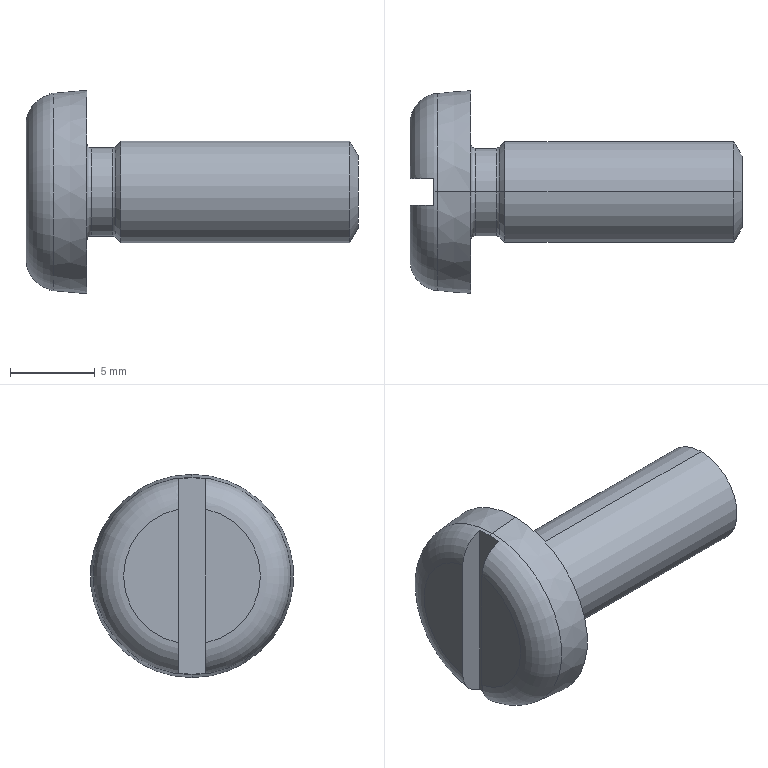Part | SolidWorks | features Fillet 2, ICE 1, LPattern 1, RevCut 1, Revolution 1 | 1 solid | 23 faces | box 19.6 x 12 x 12 mm | volume 779.516 mm3 | plane 7 | cone 6 | torus 6 | cylinder 4 | commonest cylinder face diameters 5.196 x2 6 x2
STEP:
#1=CARTESIAN_POINT('',(19.6,0.,2.134));
#2=VERTEX_POINT('',#1);
#3=CARTESIAN_POINT('',(19.6,0.,-2.134));
#4=VERTEX_POINT('',#3);
#5=CARTESIAN_POINT('',(19.6,0.,0.));
#6=DIRECTION('',(-1.,0.,0.));
#7=DIRECTION('',(0.,0.,1.));
#8=AXIS2_PLACEMENT_3D('',#5,#6,#7);
#9=CIRCLE('',#8,2.134);
#10=EDGE_CURVE('',#2,#4,#9,.T.);
#11=ORIENTED_EDGE('',*,*,#10,.T.);
#12=CARTESIAN_POINT('',(19.105,0.,-3.));
#13=VERTEX_POINT('',#12);
#14=CARTESIAN_POINT('',(19.105,0.,-3.));
#15=DIRECTION('',(-0.4959,0.,-0.8684));
#16=VECTOR('',#15,1000.);
#17=LINE('',#14,#16);
#18=EDGE_CURVE('',#4,#13,#17,.T.);
#19=ORIENTED_EDGE('',*,*,#18,.T.);
#20=CARTESIAN_POINT('',(19.105,0.,3.));
#21=VERTEX_POINT('',#20);
#22=CARTESIAN_POINT('',(19.105,0.,0.));
#23=DIRECTION('',(-1.,0.,0.));
#24=DIRECTION('',(0.,0.,1.));
#25=AXIS2_PLACEMENT_3D('',#22,#23,#24);
#26=CIRCLE('',#25,3.);
#27=EDGE_CURVE('',#21,#13,#26,.T.);
#28=ORIENTED_EDGE('',*,*,#27,.F.);
#29=CARTESIAN_POINT('',(19.105,0.,3.));
#30=DIRECTION('',(-0.4959,0.,0.8684));
#31=VECTOR('',#30,1000.);
#32=LINE('',#29,#31);
#33=EDGE_CURVE('',#2,#21,#32,.T.);
#34=ORIENTED_EDGE('',*,*,#33,.F.);
#35=EDGE_LOOP('',(#11,#19,#28,#34));
#36=FACE_OUTER_BOUND('',#35,.T.);
#37=CARTESIAN_POINT('',(19.105,0.,0.));
#38=DIRECTION('',(-1.,0.,0.));
#39=DIRECTION('',(0.,0.,1.));
#40=AXIS2_PLACEMENT_3D('',#37,#38,#39);
#41=CONICAL_SURFACE('',#40,3.,1.052);
#42=ADVANCED_FACE('',(#36),#41,.T.);
#43=CARTESIAN_POINT('',(3.6,0.,-2.848));
#44=VERTEX_POINT('',#43);
#45=CARTESIAN_POINT('',(3.6,0.,2.848));
#46=VERTEX_POINT('',#45);
#47=CARTESIAN_POINT('',(3.6,0.,0.));
#48=DIRECTION('',(-1.,0.,0.));
#49=DIRECTION('',(0.,0.,1.));
#50=AXIS2_PLACEMENT_3D('',#47,#48,#49);
#51=CIRCLE('',#50,2.848);
#52=EDGE_CURVE('',#44,#46,#51,.T.);
#53=ORIENTED_EDGE('',*,*,#52,.F.);
#54=CARTESIAN_POINT('',(3.85,0.,-2.598));
#55=VERTEX_POINT('',#54);
#56=CARTESIAN_POINT('',(3.85,0.,-2.848));
#57=DIRECTION('',(0.,1.,0.));
#58=DIRECTION('',(0.,0.,1.));
#59=AXIS2_PLACEMENT_3D('',#56,#57,#58);
#60=CIRCLE('',#59,0.25);
#61=EDGE_CURVE('',#44,#55,#60,.T.);
#62=ORIENTED_EDGE('',*,*,#61,.T.);
#63=CARTESIAN_POINT('',(3.85,0.,2.598));
#64=VERTEX_POINT('',#63);
#65=CARTESIAN_POINT('',(3.85,0.,0.));
#66=DIRECTION('',(1.,0.,0.));
#67=DIRECTION('',(0.,0.,1.));
#68=AXIS2_PLACEMENT_3D('',#65,#66,#67);
#69=CIRCLE('',#68,2.598);
#70=EDGE_CURVE('',#64,#55,#69,.T.);
#71=ORIENTED_EDGE('',*,*,#70,.F.);
#72=CARTESIAN_POINT('',(3.85,0.,2.848));
#73=DIRECTION('',(0.,-1.,0.));
#74=DIRECTION('',(0.,0.,-1.));
#75=AXIS2_PLACEMENT_3D('',#72,#73,#74);
#76=CIRCLE('',#75,0.25);
#77=EDGE_CURVE('',#46,#64,#76,.T.);
#78=ORIENTED_EDGE('',*,*,#77,.F.);
#79=EDGE_LOOP('',(#53,#62,#71,#78));
#80=FACE_OUTER_BOUND('',#79,.T.);
#81=CARTESIAN_POINT('',(3.85,0.,0.));
#82=DIRECTION('',(-1.,0.,0.));
#83=DIRECTION('',(0.,0.,1.));
#84=AXIS2_PLACEMENT_3D('',#81,#82,#83);
#85=TOROIDAL_SURFACE('',#84,2.848,0.25);
#86=ADVANCED_FACE('',(#80),#85,.F.);
#87=CARTESIAN_POINT('',(5.094,0.,-2.598));
#88=VERTEX_POINT('',#87);
#89=CARTESIAN_POINT('',(5.094,0.,2.598));
#90=VERTEX_POINT('',#89);
#91=CARTESIAN_POINT('',(5.094,0.,0.));
#92=DIRECTION('',(-1.,0.,0.));
#93=DIRECTION('',(0.,0.,1.));
#94=AXIS2_PLACEMENT_3D('',#91,#92,#93);
#95=CIRCLE('',#94,2.598);
#96=EDGE_CURVE('',#88,#90,#95,.T.);
#97=ORIENTED_EDGE('',*,*,#96,.F.);
#98=CARTESIAN_POINT('',(5.271,0.,-2.671));
#99=VERTEX_POINT('',#98);
#100=CARTESIAN_POINT('',(5.094,0.,-2.848));
#101=DIRECTION('',(0.,1.,0.));
#102=DIRECTION('',(0.,0.,1.));
#103=AXIS2_PLACEMENT_3D('',#100,#101,#102);
#104=CIRCLE('',#103,0.25);
#105=EDGE_CURVE('',#88,#99,#104,.T.);
#106=ORIENTED_EDGE('',*,*,#105,.T.);
#107=CARTESIAN_POINT('',(5.271,0.,2.671));
#108=VERTEX_POINT('',#107);
#109=CARTESIAN_POINT('',(5.271,0.,0.));
#110=DIRECTION('',(1.,0.,0.));
#111=DIRECTION('',(0.,0.,-1.));
#112=AXIS2_PLACEMENT_3D('',#109,#110,#111);
#113=CIRCLE('',#112,2.671);
#114=EDGE_CURVE('',#108,#99,#113,.T.);
#115=ORIENTED_EDGE('',*,*,#114,.F.);
#116=CARTESIAN_POINT('',(5.094,0.,2.848));
#117=DIRECTION('',(0.,-1.,0.));
#118=DIRECTION('',(0.,0.,-1.));
#119=AXIS2_PLACEMENT_3D('',#116,#117,#118);
#120=CIRCLE('',#119,0.25);
#121=EDGE_CURVE('',#90,#108,#120,.T.);
#122=ORIENTED_EDGE('',*,*,#121,.F.);
#123=EDGE_LOOP('',(#97,#106,#115,#122));
#124=FACE_OUTER_BOUND('',#123,.T.);
#125=CARTESIAN_POINT('',(5.094,0.,0.));
#126=DIRECTION('',(-1.,0.,0.));
#127=DIRECTION('',(0.,0.,1.));
#128=AXIS2_PLACEMENT_3D('',#125,#126,#127);
#129=TOROIDAL_SURFACE('',#128,2.848,0.25);
#130=ADVANCED_FACE('',(#124),#129,.F.);
#131=CARTESIAN_POINT('',(1.643,0.,-5.829));
#132=VERTEX_POINT('',#131);
#133=CARTESIAN_POINT('',(1.643,0.,5.829));
#134=VERTEX_POINT('',#133);
#135=CARTESIAN_POINT('',(1.643,0.,0.));
#136=DIRECTION('',(1.,0.,0.));
#137=DIRECTION('',(0.,0.,1.));
#138=AXIS2_PLACEMENT_3D('',#135,#136,#137);
#139=CIRCLE('',#138,5.829);
#140=EDGE_CURVE('',#132,#134,#139,.T.);
#141=ORIENTED_EDGE('',*,*,#140,.T.);
#142=CARTESIAN_POINT('',(3.6,0.,6.));
#143=VERTEX_POINT('',#142);
#144=CARTESIAN_POINT('',(3.6,0.,6.));
#145=DIRECTION('',(0.9962,0.,0.08716));
#146=VECTOR('',#145,1000.);
#147=LINE('',#144,#146);
#148=EDGE_CURVE('',#134,#143,#147,.T.);
#149=ORIENTED_EDGE('',*,*,#148,.T.);
#150=CARTESIAN_POINT('',(3.6,0.,-6.));
#151=VERTEX_POINT('',#150);
#152=CARTESIAN_POINT('',(3.6,0.,0.));
#153=DIRECTION('',(-1.,0.,0.));
#154=DIRECTION('',(0.,0.,1.));
#155=AXIS2_PLACEMENT_3D('',#152,#153,#154);
#156=CIRCLE('',#155,6.);
#157=EDGE_CURVE('',#143,#151,#156,.T.);
#158=ORIENTED_EDGE('',*,*,#157,.T.);
#159=CARTESIAN_POINT('',(3.6,0.,-6.));
#160=DIRECTION('',(0.9962,0.,-0.08716));
#161=VECTOR('',#160,1000.);
#162=LINE('',#159,#161);
#163=EDGE_CURVE('',#132,#151,#162,.T.);
#164=ORIENTED_EDGE('',*,*,#163,.F.);
#165=EDGE_LOOP('',(#141,#149,#158,#164));
#166=FACE_OUTER_BOUND('',#165,.T.);
#167=CARTESIAN_POINT('',(3.6,0.,0.));
#168=DIRECTION('',(1.,0.,0.));
#169=DIRECTION('',(0.,0.,-1.));
#170=AXIS2_PLACEMENT_3D('',#167,#168,#169);
#171=CONICAL_SURFACE('',#170,6.,0.08727);
#172=ADVANCED_FACE('',(#166),#171,.T.);
#173=CARTESIAN_POINT('',(5.094,0.,0.));
#174=DIRECTION('',(-1.,0.,0.));
#175=DIRECTION('',(0.,0.,1.));
#176=AXIS2_PLACEMENT_3D('',#173,#174,#175);
#177=CIRCLE('',#176,2.598);
#178=EDGE_CURVE('',#90,#88,#177,.T.);
#179=ORIENTED_EDGE('',*,*,#178,.T.);
#180=CARTESIAN_POINT('',(-3.442,0.,-2.598));
#181=DIRECTION('',(-1.,0.,0.));
#182=VECTOR('',#181,1000.);
#183=LINE('',#180,#182);
#184=EDGE_CURVE('',#88,#55,#183,.T.);
#185=ORIENTED_EDGE('',*,*,#184,.T.);
#186=CARTESIAN_POINT('',(3.85,0.,0.));
#187=DIRECTION('',(1.,0.,0.));
#188=DIRECTION('',(0.,0.,1.));
#189=AXIS2_PLACEMENT_3D('',#186,#187,#188);
#190=CIRCLE('',#189,2.598);
#191=EDGE_CURVE('',#55,#64,#190,.T.);
#192=ORIENTED_EDGE('',*,*,#191,.T.);
#193=CARTESIAN_POINT('',(-3.442,0.,2.598));
#194=DIRECTION('',(-1.,0.,0.));
#195=VECTOR('',#194,1000.);
#196=LINE('',#193,#195);
#197=EDGE_CURVE('',#90,#64,#196,.T.);
#198=ORIENTED_EDGE('',*,*,#197,.F.);
#199=EDGE_LOOP('',(#179,#185,#192,#198));
#200=FACE_OUTER_BOUND('',#199,.T.);
#201=CARTESIAN_POINT('',(-3.442,0.,0.));
#202=DIRECTION('',(-1.,0.,0.));
#203=DIRECTION('',(0.,0.,1.));
#204=AXIS2_PLACEMENT_3D('',#201,#202,#203);
#205=CYLINDRICAL_SURFACE('',#204,2.598);
#206=ADVANCED_FACE('',(#200),#205,.T.);
#207=CARTESIAN_POINT('',(5.271,0.,0.));
#208=DIRECTION('',(1.,0.,0.));
#209=DIRECTION('',(0.,0.,-1.));
#210=AXIS2_PLACEMENT_3D('',#207,#208,#209);
#211=CIRCLE('',#210,2.671);
#212=EDGE_CURVE('',#99,#108,#211,.T.);
#213=ORIENTED_EDGE('',*,*,#212,.T.);
#214=CARTESIAN_POINT('',(5.6,0.,3.));
#215=VERTEX_POINT('',#214);
#216=CARTESIAN_POINT('',(5.6,0.,3.));
#217=DIRECTION('',(0.7071,0.,0.7071));
#218=VECTOR('',#217,1000.);
#219=LINE('',#216,#218);
#220=EDGE_CURVE('',#108,#215,#219,.T.);
#221=ORIENTED_EDGE('',*,*,#220,.T.);
#222=CARTESIAN_POINT('',(5.6,0.,-3.));
#223=VERTEX_POINT('',#222);
#224=CARTESIAN_POINT('',(5.6,0.,0.));
#225=DIRECTION('',(-1.,0.,0.));
#226=DIRECTION('',(0.,0.,1.));
#227=AXIS2_PLACEMENT_3D('',#224,#225,#226);
#228=CIRCLE('',#227,3.);
#229=EDGE_CURVE('',#215,#223,#228,.T.);
#230=ORIENTED_EDGE('',*,*,#229,.T.);
#231=CARTESIAN_POINT('',(5.6,0.,-3.));
#232=DIRECTION('',(0.7071,0.,-0.7071));
#233=VECTOR('',#232,1000.);
#234=LINE('',#231,#233);
#235=EDGE_CURVE('',#99,#223,#234,.T.);
#236=ORIENTED_EDGE('',*,*,#235,.F.);
#237=EDGE_LOOP('',(#213,#221,#230,#236));
#238=FACE_OUTER_BOUND('',#237,.T.);
#239=CARTESIAN_POINT('',(5.6,0.,0.));
#240=DIRECTION('',(1.,0.,0.));
#241=DIRECTION('',(0.,0.,-1.));
#242=AXIS2_PLACEMENT_3D('',#239,#240,#241);
#243=CONICAL_SURFACE('',#242,3.,0.7854);
#244=ADVANCED_FACE('',(#238),#243,.T.);
#245=CARTESIAN_POINT('',(1.4,0.8,5.735));
#246=VERTEX_POINT('',#245);
#247=CARTESIAN_POINT('',(1.4,0.,5.791));
#248=VERTEX_POINT('',#247);
#249=CARTESIAN_POINT('',(1.4,0.,0.));
#250=DIRECTION('',(1.,0.,0.));
#251=DIRECTION('',(0.,0.,1.));
#252=AXIS2_PLACEMENT_3D('',#249,#250,#251);
#253=CIRCLE('',#252,5.791);
#254=EDGE_CURVE('',#246,#248,#253,.T.);
#255=ORIENTED_EDGE('',*,*,#254,.T.);
#256=CARTESIAN_POINT('',(1.8,0.,4.036));
#257=DIRECTION('',(0.,1.,0.));
#258=DIRECTION('',(0.,0.,1.));
#259=AXIS2_PLACEMENT_3D('',#256,#257,#258);
#260=CIRCLE('',#259,1.8);
#261=EDGE_CURVE('',#248,#134,#260,.T.);
#262=ORIENTED_EDGE('',*,*,#261,.T.);
#263=ORIENTED_EDGE('',*,*,#140,.F.);
#264=CARTESIAN_POINT('',(1.4,0.,-5.791));
#265=VERTEX_POINT('',#264);
#266=CARTESIAN_POINT('',(1.8,0.,-4.036));
#267=DIRECTION('',(0.,-1.,0.));
#268=DIRECTION('',(0.,0.,-1.));
#269=AXIS2_PLACEMENT_3D('',#266,#267,#268);
#270=CIRCLE('',#269,1.8);
#271=EDGE_CURVE('',#265,#132,#270,.T.);
#272=ORIENTED_EDGE('',*,*,#271,.F.);
#273=CARTESIAN_POINT('',(1.4,0.8,-5.735));
#274=VERTEX_POINT('',#273);
#275=CARTESIAN_POINT('',(1.4,0.,0.));
#276=DIRECTION('',(1.,0.,0.));
#277=DIRECTION('',(0.,0.,1.));
#278=AXIS2_PLACEMENT_3D('',#275,#276,#277);
#279=CIRCLE('',#278,5.791);
#280=EDGE_CURVE('',#265,#274,#279,.T.);
#281=ORIENTED_EDGE('',*,*,#280,.T.);
#282=CARTESIAN_POINT('',(0.,0.8,-3.956));
#283=VERTEX_POINT('',#282);
#284=CARTESIAN_POINT('',(1.4,0.8,-5.735));
#285=CARTESIAN_POINT('',(1.203,0.8,-5.69));
#286=CARTESIAN_POINT('',(1.011,0.8,-5.609));
#287=CARTESIAN_POINT('',(0.6651,0.8,-5.389));
#288=CARTESIAN_POINT('',(0.5144,0.8,-5.251));
#289=CARTESIAN_POINT('',(0.2624,0.8,-4.929));
#290=CARTESIAN_POINT('',(0.1653,0.8,-4.749));
#291=CARTESIAN_POINT('',(0.03314,0.8,-4.362));
#292=CARTESIAN_POINT('',(0.,0.8,-4.16));
#293=CARTESIAN_POINT('',(0.,0.8,-3.956));
#294=B_SPLINE_CURVE_WITH_KNOTS('',3,(#284,#285,#286,#287,#288,#289,#290,#291,#292,#293),.UNSPECIFIED.,.F.,.F.,(4,2,2,2,4),(0.01073,0.01134,0.01195,0.01255,0.01316),.UNSPECIFIED.);
#295=EDGE_CURVE('',#274,#283,#294,.T.);
#296=ORIENTED_EDGE('',*,*,#295,.T.);
#297=CARTESIAN_POINT('',(0.,0.8,3.956));
#298=VERTEX_POINT('',#297);
#299=CARTESIAN_POINT('',(0.,0.,0.));
#300=DIRECTION('',(-1.,0.,0.));
#301=DIRECTION('',(0.,0.,-1.));
#302=AXIS2_PLACEMENT_3D('',#299,#300,#301);
#303=CIRCLE('',#302,4.036);
#304=EDGE_CURVE('',#298,#283,#303,.T.);
#305=ORIENTED_EDGE('',*,*,#304,.F.);
#306=CARTESIAN_POINT('',(0.,0.8,3.956));
#307=CARTESIAN_POINT('',(0.,0.8,4.057));
#308=CARTESIAN_POINT('',(0.008433,0.8,4.16));
#309=CARTESIAN_POINT('',(0.04179,0.8,4.361));
#310=CARTESIAN_POINT('',(0.06654,0.8,4.46));
#311=CARTESIAN_POINT('',(0.165,0.8,4.748));
#312=CARTESIAN_POINT('',(0.2638,0.8,4.931));
#313=CARTESIAN_POINT('',(0.5139,0.8,5.25));
#314=CARTESIAN_POINT('',(0.6679,0.8,5.391));
#315=CARTESIAN_POINT('',(1.01,0.8,5.609));
#316=CARTESIAN_POINT('',(1.202,0.8,5.69));
#317=CARTESIAN_POINT('',(1.4,0.8,5.735));
#318=B_SPLINE_CURVE_WITH_KNOTS('',3,(#306,#307,#308,#309,#310,#311,#312,#313,#314,#315,#316,#317),.UNSPECIFIED.,.F.,.F.,(4,2,2,2,2,4),(0.001725,0.002029,0.002333,0.002941,0.003549,0.004157),.UNSPECIFIED.);
#319=EDGE_CURVE('',#298,#246,#318,.T.);
#320=ORIENTED_EDGE('',*,*,#319,.T.);
#321=EDGE_LOOP('',(#255,#262,#263,#272,#281,#296,#305,#320));
#322=FACE_OUTER_BOUND('',#321,.T.);
#323=CARTESIAN_POINT('',(1.8,0.,0.));
#324=DIRECTION('',(1.,0.,0.));
#325=DIRECTION('',(0.,0.,-1.));
#326=AXIS2_PLACEMENT_3D('',#323,#324,#325);
#327=TOROIDAL_SURFACE('',#326,4.036,1.8);
#328=ADVANCED_FACE('',(#322),#327,.T.);
#329=ORIENTED_EDGE('',*,*,#27,.T.);
#330=CARTESIAN_POINT('',(-3.442,0.,-3.));
#331=DIRECTION('',(-1.,0.,0.));
#332=VECTOR('',#331,1000.);
#333=LINE('',#330,#332);
#334=EDGE_CURVE('',#13,#223,#333,.T.);
#335=ORIENTED_EDGE('',*,*,#334,.T.);
#336=ORIENTED_EDGE('',*,*,#229,.F.);
#337=CARTESIAN_POINT('',(-3.442,0.,3.));
#338=DIRECTION('',(-1.,0.,0.));
#339=VECTOR('',#338,1000.);
#340=LINE('',#337,#339);
#341=EDGE_CURVE('',#21,#215,#340,.T.);
#342=ORIENTED_EDGE('',*,*,#341,.F.);
#343=EDGE_LOOP('',(#329,#335,#336,#342));
#344=FACE_OUTER_BOUND('',#343,.T.);
#345=CARTESIAN_POINT('',(-3.442,0.,0.));
#346=DIRECTION('',(-1.,0.,0.));
#347=DIRECTION('',(0.,0.,1.));
#348=AXIS2_PLACEMENT_3D('',#345,#346,#347);
#349=CYLINDRICAL_SURFACE('',#348,3.);
#350=ADVANCED_FACE('',(#344),#349,.T.);
#351=ORIENTED_EDGE('',*,*,#334,.F.);
#352=CARTESIAN_POINT('',(19.105,0.,0.));
#353=DIRECTION('',(-1.,0.,0.));
#354=DIRECTION('',(0.,0.,1.));
#355=AXIS2_PLACEMENT_3D('',#352,#353,#354);
#356=CIRCLE('',#355,3.);
#357=EDGE_CURVE('',#13,#21,#356,.T.);
#358=ORIENTED_EDGE('',*,*,#357,.T.);
#359=ORIENTED_EDGE('',*,*,#341,.T.);
#360=CARTESIAN_POINT('',(5.6,0.,0.));
#361=DIRECTION('',(-1.,0.,0.));
#362=DIRECTION('',(0.,0.,1.));
#363=AXIS2_PLACEMENT_3D('',#360,#361,#362);
#364=CIRCLE('',#363,3.);
#365=EDGE_CURVE('',#223,#215,#364,.T.);
#366=ORIENTED_EDGE('',*,*,#365,.F.);
#367=EDGE_LOOP('',(#351,#358,#359,#366));
#368=FACE_OUTER_BOUND('',#367,.T.);
#369=CARTESIAN_POINT('',(-3.442,0.,0.));
#370=DIRECTION('',(-1.,0.,0.));
#371=DIRECTION('',(0.,0.,1.));
#372=AXIS2_PLACEMENT_3D('',#369,#370,#371);
#373=CYLINDRICAL_SURFACE('',#372,3.);
#374=ADVANCED_FACE('',(#368),#373,.T.);
#375=CARTESIAN_POINT('',(0.,-0.8,3.956));
#376=VERTEX_POINT('',#375);
#377=CARTESIAN_POINT('',(0.,-0.8,-3.956));
#378=VERTEX_POINT('',#377);
#379=CARTESIAN_POINT('',(0.,-0.8,-6.));
#380=DIRECTION('',(0.,0.,-1.));
#381=VECTOR('',#380,1000.);
#382=LINE('',#379,#381);
#383=EDGE_CURVE('',#376,#378,#382,.T.);
#384=ORIENTED_EDGE('',*,*,#383,.T.);
#385=CARTESIAN_POINT('',(0.,0.,0.));
#386=DIRECTION('',(-1.,0.,0.));
#387=DIRECTION('',(0.,0.,-1.));
#388=AXIS2_PLACEMENT_3D('',#385,#386,#387);
#389=CIRCLE('',#388,4.036);
#390=EDGE_CURVE('',#378,#376,#389,.T.);
#391=ORIENTED_EDGE('',*,*,#390,.T.);
#392=EDGE_LOOP('',(#384,#391));
#393=FACE_OUTER_BOUND('',#392,.T.);
#394=CARTESIAN_POINT('',(0.,5.685,0.));
#395=DIRECTION('',(1.,0.,0.));
#396=DIRECTION('',(0.,0.,-1.));
#397=AXIS2_PLACEMENT_3D('',#394,#395,#396);
#398=PLANE('',#397);
#399=ADVANCED_FACE('',(#393),#398,.F.);
#400=CARTESIAN_POINT('',(0.,0.8,-6.));
#401=DIRECTION('',(0.,0.,1.));
#402=VECTOR('',#401,1000.);
#403=LINE('',#400,#402);
#404=EDGE_CURVE('',#283,#298,#403,.T.);
#405=ORIENTED_EDGE('',*,*,#404,.T.);
#406=ORIENTED_EDGE('',*,*,#304,.T.);
#407=EDGE_LOOP('',(#405,#406));
#408=FACE_OUTER_BOUND('',#407,.T.);
#409=CARTESIAN_POINT('',(0.,5.685,0.));
#410=DIRECTION('',(1.,0.,0.));
#411=DIRECTION('',(0.,0.,-1.));
#412=AXIS2_PLACEMENT_3D('',#409,#410,#411);
#413=PLANE('',#412);
#414=ADVANCED_FACE('',(#408),#413,.F.);
#415=ORIENTED_EDGE('',*,*,#261,.F.);
#416=CARTESIAN_POINT('',(1.4,-0.8,5.735));
#417=VERTEX_POINT('',#416);
#418=CARTESIAN_POINT('',(1.4,0.,0.));
#419=DIRECTION('',(1.,0.,0.));
#420=DIRECTION('',(0.,0.,1.));
#421=AXIS2_PLACEMENT_3D('',#418,#419,#420);
#422=CIRCLE('',#421,5.791);
#423=EDGE_CURVE('',#248,#417,#422,.T.);
#424=ORIENTED_EDGE('',*,*,#423,.T.);
#425=CARTESIAN_POINT('',(1.4,-0.8,5.735));
#426=CARTESIAN_POINT('',(1.2,-0.8,5.689));
#427=CARTESIAN_POINT('',(1.012,-0.8,5.61));
#428=CARTESIAN_POINT('',(0.6661,-0.8,5.389));
#429=CARTESIAN_POINT('',(0.5155,-0.8,5.252));
#430=CARTESIAN_POINT('',(0.2624,-0.8,4.929));
#431=CARTESIAN_POINT('',(0.1658,-0.8,4.75));
#432=CARTESIAN_POINT('',(0.03297,-0.8,4.361));
#433=CARTESIAN_POINT('',(0.,-0.8,4.161));
#434=CARTESIAN_POINT('',(0.,-0.8,3.956));
#435=B_SPLINE_CURVE_WITH_KNOTS('',3,(#425,#426,#427,#428,#429,#430,#431,#432,#433,#434),.UNSPECIFIED.,.F.,.F.,(4,2,2,2,4),(0.00724,0.007848,0.008457,0.009065,0.009674),.UNSPECIFIED.);
#436=EDGE_CURVE('',#417,#376,#435,.T.);
#437=ORIENTED_EDGE('',*,*,#436,.T.);
#438=ORIENTED_EDGE('',*,*,#390,.F.);
#439=CARTESIAN_POINT('',(1.4,-0.8,-5.735));
#440=VERTEX_POINT('',#439);
#441=CARTESIAN_POINT('',(0.,-0.8,-3.956));
#442=CARTESIAN_POINT('',(0.,-0.8,-4.057));
#443=CARTESIAN_POINT('',(0.008456,-0.8,-4.16));
#444=CARTESIAN_POINT('',(0.04165,-0.8,-4.361));
#445=CARTESIAN_POINT('',(0.0663,-0.8,-4.459));
#446=CARTESIAN_POINT('',(0.1319,-0.8,-4.651));
#447=CARTESIAN_POINT('',(0.1733,-0.8,-4.746));
#448=CARTESIAN_POINT('',(0.27,-0.8,-4.925));
#449=CARTESIAN_POINT('',(0.3254,-0.8,-5.009));
#450=CARTESIAN_POINT('',(0.5128,-0.8,-5.249));
#451=CARTESIAN_POINT('',(0.6672,-0.8,-5.39));
#452=CARTESIAN_POINT('',(1.012,-0.8,-5.61));
#453=CARTESIAN_POINT('',(1.201,-0.8,-5.689));
#454=CARTESIAN_POINT('',(1.4,-0.8,-5.735));
#455=B_SPLINE_CURVE_WITH_KNOTS('',3,(#441,#442,#443,#444,#445,#446,#447,#448,#449,#450,#451,#452,#453,#454),.UNSPECIFIED.,.F.,.F.,(4,2,2,2,2,2,4),(0.009623,0.009926,0.01023,0.01053,0.01084,0.01145,0.01205),.UNSPECIFIED.);
#456=EDGE_CURVE('',#378,#440,#455,.T.);
#457=ORIENTED_EDGE('',*,*,#456,.T.);
#458=CARTESIAN_POINT('',(1.4,0.,0.));
#459=DIRECTION('',(1.,0.,0.));
#460=DIRECTION('',(0.,0.,1.));
#461=AXIS2_PLACEMENT_3D('',#458,#459,#460);
#462=CIRCLE('',#461,5.791);
#463=EDGE_CURVE('',#440,#265,#462,.T.);
#464=ORIENTED_EDGE('',*,*,#463,.T.);
#465=ORIENTED_EDGE('',*,*,#271,.T.);
#466=CARTESIAN_POINT('',(1.643,0.,0.));
#467=DIRECTION('',(1.,0.,0.));
#468=DIRECTION('',(0.,0.,1.));
#469=AXIS2_PLACEMENT_3D('',#466,#467,#468);
#470=CIRCLE('',#469,5.829);
#471=EDGE_CURVE('',#134,#132,#470,.T.);
#472=ORIENTED_EDGE('',*,*,#471,.F.);
#473=EDGE_LOOP('',(#415,#424,#437,#438,#457,#464,#465,#472));
#474=FACE_OUTER_BOUND('',#473,.T.);
#475=CARTESIAN_POINT('',(1.8,0.,0.));
#476=DIRECTION('',(1.,0.,0.));
#477=DIRECTION('',(0.,0.,-1.));
#478=AXIS2_PLACEMENT_3D('',#475,#476,#477);
#479=TOROIDAL_SURFACE('',#478,4.036,1.8);
#480=ADVANCED_FACE('',(#474),#479,.T.);
#481=ORIENTED_EDGE('',*,*,#220,.F.);
#482=ORIENTED_EDGE('',*,*,#114,.T.);
#483=ORIENTED_EDGE('',*,*,#235,.T.);
#484=ORIENTED_EDGE('',*,*,#365,.T.);
#485=EDGE_LOOP('',(#481,#482,#483,#484));
#486=FACE_OUTER_BOUND('',#485,.T.);
#487=CARTESIAN_POINT('',(5.6,0.,0.));
#488=DIRECTION('',(1.,0.,0.));
#489=DIRECTION('',(0.,0.,-1.));
#490=AXIS2_PLACEMENT_3D('',#487,#488,#489);
#491=CONICAL_SURFACE('',#490,3.,0.7854);
#492=ADVANCED_FACE('',(#486),#491,.T.);
#493=ORIENTED_EDGE('',*,*,#184,.F.);
#494=ORIENTED_EDGE('',*,*,#96,.T.);
#495=ORIENTED_EDGE('',*,*,#197,.T.);
#496=ORIENTED_EDGE('',*,*,#70,.T.);
#497=EDGE_LOOP('',(#493,#494,#495,#496));
#498=FACE_OUTER_BOUND('',#497,.T.);
#499=CARTESIAN_POINT('',(-3.442,0.,0.));
#500=DIRECTION('',(-1.,0.,0.));
#501=DIRECTION('',(0.,0.,1.));
#502=AXIS2_PLACEMENT_3D('',#499,#500,#501);
#503=CYLINDRICAL_SURFACE('',#502,2.598);
#504=ADVANCED_FACE('',(#498),#503,.T.);
#505=CARTESIAN_POINT('',(3.6,0.,0.));
#506=DIRECTION('',(-1.,0.,0.));
#507=DIRECTION('',(0.,0.,1.));
#508=AXIS2_PLACEMENT_3D('',#505,#506,#507);
#509=CIRCLE('',#508,2.848);
#510=EDGE_CURVE('',#46,#44,#509,.T.);
#511=ORIENTED_EDGE('',*,*,#510,.T.);
#512=ORIENTED_EDGE('',*,*,#52,.T.);
#513=EDGE_LOOP('',(#511,#512));
#514=FACE_BOUND('',#513,.T.);
#515=CARTESIAN_POINT('',(3.6,0.,0.));
#516=DIRECTION('',(-1.,0.,0.));
#517=DIRECTION('',(0.,0.,1.));
#518=AXIS2_PLACEMENT_3D('',#515,#516,#517);
#519=CIRCLE('',#518,6.);
#520=EDGE_CURVE('',#151,#143,#519,.T.);
#521=ORIENTED_EDGE('',*,*,#520,.F.);
#522=ORIENTED_EDGE('',*,*,#157,.F.);
#523=EDGE_LOOP('',(#521,#522));
#524=FACE_OUTER_BOUND('',#523,.T.);
#525=CARTESIAN_POINT('',(3.6,6.,0.));
#526=DIRECTION('',(-1.,0.,0.));
#527=DIRECTION('',(0.,0.,1.));
#528=AXIS2_PLACEMENT_3D('',#525,#526,#527);
#529=PLANE('',#528);
#530=ADVANCED_FACE('',(#514,#524),#529,.F.);
#531=ORIENTED_EDGE('',*,*,#148,.F.);
#532=ORIENTED_EDGE('',*,*,#471,.T.);
#533=ORIENTED_EDGE('',*,*,#163,.T.);
#534=ORIENTED_EDGE('',*,*,#520,.T.);
#535=EDGE_LOOP('',(#531,#532,#533,#534));
#536=FACE_OUTER_BOUND('',#535,.T.);
#537=CARTESIAN_POINT('',(3.6,0.,0.));
#538=DIRECTION('',(1.,0.,0.));
#539=DIRECTION('',(0.,0.,-1.));
#540=AXIS2_PLACEMENT_3D('',#537,#538,#539);
#541=CONICAL_SURFACE('',#540,6.,0.08727);
#542=ADVANCED_FACE('',(#536),#541,.T.);
#543=ORIENTED_EDGE('',*,*,#105,.F.);
#544=ORIENTED_EDGE('',*,*,#178,.F.);
#545=ORIENTED_EDGE('',*,*,#121,.T.);
#546=ORIENTED_EDGE('',*,*,#212,.F.);
#547=EDGE_LOOP('',(#543,#544,#545,#546));
#548=FACE_OUTER_BOUND('',#547,.T.);
#549=CARTESIAN_POINT('',(5.094,0.,0.));
#550=DIRECTION('',(-1.,0.,0.));
#551=DIRECTION('',(0.,0.,1.));
#552=AXIS2_PLACEMENT_3D('',#549,#550,#551);
#553=TOROIDAL_SURFACE('',#552,2.848,0.25);
#554=ADVANCED_FACE('',(#548),#553,.F.);
#555=ORIENTED_EDGE('',*,*,#61,.F.);
#556=ORIENTED_EDGE('',*,*,#510,.F.);
#557=ORIENTED_EDGE('',*,*,#77,.T.);
#558=ORIENTED_EDGE('',*,*,#191,.F.);
#559=EDGE_LOOP('',(#555,#556,#557,#558));
#560=FACE_OUTER_BOUND('',#559,.T.);
#561=CARTESIAN_POINT('',(3.85,0.,0.));
#562=DIRECTION('',(-1.,0.,0.));
#563=DIRECTION('',(0.,0.,1.));
#564=AXIS2_PLACEMENT_3D('',#561,#562,#563);
#565=TOROIDAL_SURFACE('',#564,2.848,0.25);
#566=ADVANCED_FACE('',(#560),#565,.F.);
#567=ORIENTED_EDGE('',*,*,#383,.F.);
#568=ORIENTED_EDGE('',*,*,#436,.F.);
#569=CARTESIAN_POINT('',(1.4,-0.8,-6.));
#570=DIRECTION('',(0.,0.,-1.));
#571=VECTOR('',#570,1000.);
#572=LINE('',#569,#571);
#573=EDGE_CURVE('',#417,#440,#572,.T.);
#574=ORIENTED_EDGE('',*,*,#573,.T.);
#575=ORIENTED_EDGE('',*,*,#456,.F.);
#576=EDGE_LOOP('',(#567,#568,#574,#575));
#577=FACE_OUTER_BOUND('',#576,.T.);
#578=CARTESIAN_POINT('',(1.4,-0.8,-6.));
#579=DIRECTION('',(0.,1.,0.));
#580=DIRECTION('',(0.,0.,1.));
#581=AXIS2_PLACEMENT_3D('',#578,#579,#580);
#582=PLANE('',#581);
#583=ADVANCED_FACE('',(#577),#582,.T.);
#584=CARTESIAN_POINT('',(1.4,0.8,-6.));
#585=DIRECTION('',(0.,0.,1.));
#586=VECTOR('',#585,1000.);
#587=LINE('',#584,#586);
#588=EDGE_CURVE('',#274,#246,#587,.T.);
#589=ORIENTED_EDGE('',*,*,#588,.T.);
#590=ORIENTED_EDGE('',*,*,#319,.F.);
#591=ORIENTED_EDGE('',*,*,#404,.F.);
#592=ORIENTED_EDGE('',*,*,#295,.F.);
#593=EDGE_LOOP('',(#589,#590,#591,#592));
#594=FACE_OUTER_BOUND('',#593,.T.);
#595=CARTESIAN_POINT('',(1.4,0.8,-6.));
#596=DIRECTION('',(0.,-1.,0.));
#597=DIRECTION('',(0.,0.,-1.));
#598=AXIS2_PLACEMENT_3D('',#595,#596,#597);
#599=PLANE('',#598);
#600=ADVANCED_FACE('',(#594),#599,.T.);
#601=ORIENTED_EDGE('',*,*,#573,.F.);
#602=ORIENTED_EDGE('',*,*,#423,.F.);
#603=ORIENTED_EDGE('',*,*,#254,.F.);
#604=ORIENTED_EDGE('',*,*,#588,.F.);
#605=ORIENTED_EDGE('',*,*,#280,.F.);
#606=ORIENTED_EDGE('',*,*,#463,.F.);
#607=EDGE_LOOP('',(#601,#602,#603,#604,#605,#606));
#608=FACE_OUTER_BOUND('',#607,.T.);
#609=CARTESIAN_POINT('',(1.4,-0.8,6.));
#610=DIRECTION('',(-1.,0.,0.));
#611=DIRECTION('',(0.,0.,1.));
#612=AXIS2_PLACEMENT_3D('',#609,#610,#611);
#613=PLANE('',#612);
#614=ADVANCED_FACE('',(#608),#613,.T.);
#615=ORIENTED_EDGE('',*,*,#18,.F.);
#616=CARTESIAN_POINT('',(19.6,0.,0.));
#617=DIRECTION('',(-1.,0.,0.));
#618=DIRECTION('',(0.,0.,1.));
#619=AXIS2_PLACEMENT_3D('',#616,#617,#618);
#620=CIRCLE('',#619,2.134);
#621=EDGE_CURVE('',#4,#2,#620,.T.);
#622=ORIENTED_EDGE('',*,*,#621,.T.);
#623=ORIENTED_EDGE('',*,*,#33,.T.);
#624=ORIENTED_EDGE('',*,*,#357,.F.);
#625=EDGE_LOOP('',(#615,#622,#623,#624));
#626=FACE_OUTER_BOUND('',#625,.T.);
#627=CARTESIAN_POINT('',(19.105,0.,0.));
#628=DIRECTION('',(-1.,0.,0.));
#629=DIRECTION('',(0.,0.,1.));
#630=AXIS2_PLACEMENT_3D('',#627,#628,#629);
#631=CONICAL_SURFACE('',#630,3.,1.052);
#632=ADVANCED_FACE('',(#626),#631,.T.);
#633=ORIENTED_EDGE('',*,*,#10,.F.);
#634=ORIENTED_EDGE('',*,*,#621,.F.);
#635=EDGE_LOOP('',(#633,#634));
#636=FACE_OUTER_BOUND('',#635,.T.);
#637=CARTESIAN_POINT('',(19.6,0.,0.));
#638=DIRECTION('',(-1.,0.,0.));
#639=DIRECTION('',(0.,0.,1.));
#640=AXIS2_PLACEMENT_3D('',#637,#638,#639);
#641=PLANE('',#640);
#642=ADVANCED_FACE('',(#636),#641,.F.);
#643=CLOSED_SHELL('',(#42,#86,#130,#172,#206,#244,#328,#350,#374,#399,#414,#480,#492,#504,#530,#542,#554,#566,#583,#600,#614,#632,#642));
#644=MANIFOLD_SOLID_BREP('',#643);
#645=CARTESIAN_POINT('',(0.,0.,0.));
#646=DIRECTION('',(0.,0.,1.));
#647=DIRECTION('',(1.,0.,0.));
#648=AXIS2_PLACEMENT_3D('',#645,#646,#647);
#649=(LENGTH_UNIT()NAMED_UNIT(*)SI_UNIT(.MILLI.,.METRE.));
#650=UNCERTAINTY_MEASURE_WITH_UNIT(LENGTH_MEASURE(0.00001),#649,'','');
#651=(NAMED_UNIT(*)PLANE_ANGLE_UNIT()SI_UNIT($,.RADIAN.));
#652=(NAMED_UNIT(*)SI_UNIT($,.STERADIAN.)SOLID_ANGLE_UNIT());
#653=(GEOMETRIC_REPRESENTATION_CONTEXT(3)GLOBAL_UNCERTAINTY_ASSIGNED_CONTEXT((#650))GLOBAL_UNIT_ASSIGNED_CONTEXT((#649,#651,#652))REPRESENTATION_CONTEXT('',''));
#654=ADVANCED_BREP_SHAPE_REPRESENTATION('',(#644,#648),#653);